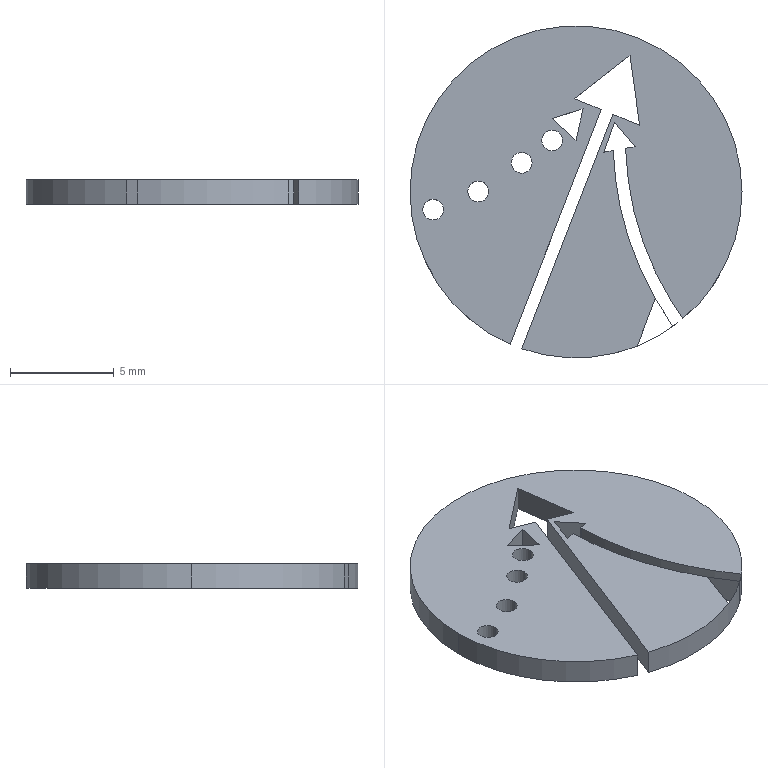Part | STEP file | Part 11_1 | 1 solid | 31 faces | box 16 x 16 x 1.2 mm | volume 213.852 mm3 | plane 17 | cylinder 12 | spline 2 | commonest cylinder face diameters 1 x8 16 x4
STEP:
#1=CARTESIAN_POINT('',(-6.382,-0.8597,1.2));
#2=VERTEX_POINT('',#1);
#3=CARTESIAN_POINT('',(-7.382,-0.8597,1.2));
#4=VERTEX_POINT('',#3);
#5=CARTESIAN_POINT('',(-6.882,-0.8597,1.2));
#6=DIRECTION('',(0.,0.,-1.));
#7=DIRECTION('',(-1.,0.,0.));
#8=AXIS2_PLACEMENT_3D('',#5,#6,#7);
#9=CIRCLE('',#8,0.5);
#10=EDGE_CURVE('',#2,#4,#9,.T.);
#11=ORIENTED_EDGE('',*,*,#10,.F.);
#12=CARTESIAN_POINT('',(-6.382,-0.8597,0.));
#13=VERTEX_POINT('',#12);
#14=CARTESIAN_POINT('',(-6.382,-0.8597,10.));
#15=DIRECTION('',(0.,0.,-1.));
#16=VECTOR('',#15,1000.);
#17=LINE('',#14,#16);
#18=EDGE_CURVE('',#2,#13,#17,.T.);
#19=ORIENTED_EDGE('',*,*,#18,.T.);
#20=CARTESIAN_POINT('',(-7.382,-0.8597,0.));
#21=VERTEX_POINT('',#20);
#22=CARTESIAN_POINT('',(-6.882,-0.8597,0.));
#23=DIRECTION('',(0.,0.,1.));
#24=DIRECTION('',(-1.,0.,0.));
#25=AXIS2_PLACEMENT_3D('',#22,#23,#24);
#26=CIRCLE('',#25,0.5);
#27=EDGE_CURVE('',#21,#13,#26,.T.);
#28=ORIENTED_EDGE('',*,*,#27,.F.);
#29=CARTESIAN_POINT('',(-7.382,-0.8597,10.));
#30=DIRECTION('',(0.,0.,-1.));
#31=VECTOR('',#30,1000.);
#32=LINE('',#29,#31);
#33=EDGE_CURVE('',#4,#21,#32,.T.);
#34=ORIENTED_EDGE('',*,*,#33,.F.);
#35=EDGE_LOOP('',(#11,#19,#28,#34));
#36=FACE_OUTER_BOUND('',#35,.T.);
#37=CARTESIAN_POINT('',(-6.882,-0.8597,10.));
#38=DIRECTION('',(0.,0.,-1.));
#39=DIRECTION('',(-1.,0.,0.));
#40=AXIS2_PLACEMENT_3D('',#37,#38,#39);
#41=CYLINDRICAL_SURFACE('',#40,0.5);
#42=ADVANCED_FACE('',(#36),#41,.F.);
#43=CARTESIAN_POINT('',(-2.114,1.401,1.2));
#44=VERTEX_POINT('',#43);
#45=CARTESIAN_POINT('',(-3.114,1.401,1.2));
#46=VERTEX_POINT('',#45);
#47=CARTESIAN_POINT('',(-2.614,1.401,1.2));
#48=DIRECTION('',(0.,0.,-1.));
#49=DIRECTION('',(-1.,0.,0.));
#50=AXIS2_PLACEMENT_3D('',#47,#48,#49);
#51=CIRCLE('',#50,0.5);
#52=EDGE_CURVE('',#44,#46,#51,.T.);
#53=ORIENTED_EDGE('',*,*,#52,.F.);
#54=CARTESIAN_POINT('',(-2.114,1.401,0.));
#55=VERTEX_POINT('',#54);
#56=CARTESIAN_POINT('',(-2.114,1.401,10.));
#57=DIRECTION('',(0.,0.,-1.));
#58=VECTOR('',#57,1000.);
#59=LINE('',#56,#58);
#60=EDGE_CURVE('',#44,#55,#59,.T.);
#61=ORIENTED_EDGE('',*,*,#60,.T.);
#62=CARTESIAN_POINT('',(-3.114,1.401,0.));
#63=VERTEX_POINT('',#62);
#64=CARTESIAN_POINT('',(-2.614,1.401,0.));
#65=DIRECTION('',(0.,0.,1.));
#66=DIRECTION('',(-1.,0.,0.));
#67=AXIS2_PLACEMENT_3D('',#64,#65,#66);
#68=CIRCLE('',#67,0.5);
#69=EDGE_CURVE('',#63,#55,#68,.T.);
#70=ORIENTED_EDGE('',*,*,#69,.F.);
#71=CARTESIAN_POINT('',(-3.114,1.401,10.));
#72=DIRECTION('',(0.,0.,-1.));
#73=VECTOR('',#72,1000.);
#74=LINE('',#71,#73);
#75=EDGE_CURVE('',#46,#63,#74,.T.);
#76=ORIENTED_EDGE('',*,*,#75,.F.);
#77=EDGE_LOOP('',(#53,#61,#70,#76));
#78=FACE_OUTER_BOUND('',#77,.T.);
#79=CARTESIAN_POINT('',(-2.614,1.401,10.));
#80=DIRECTION('',(0.,0.,-1.));
#81=DIRECTION('',(-1.,0.,0.));
#82=AXIS2_PLACEMENT_3D('',#79,#80,#81);
#83=CYLINDRICAL_SURFACE('',#82,0.5);
#84=ADVANCED_FACE('',(#78),#83,.F.);
#85=CARTESIAN_POINT('',(8.,0.,1.2));
#86=VERTEX_POINT('',#85);
#87=CARTESIAN_POINT('',(-8.,0.,1.2));
#88=VERTEX_POINT('',#87);
#89=CARTESIAN_POINT('',(0.,0.,1.2));
#90=DIRECTION('',(0.,0.,1.));
#91=DIRECTION('',(-1.,0.,0.));
#92=AXIS2_PLACEMENT_3D('',#89,#90,#91);
#93=CIRCLE('',#92,8.);
#94=EDGE_CURVE('',#86,#88,#93,.T.);
#95=ORIENTED_EDGE('',*,*,#94,.F.);
#96=CARTESIAN_POINT('',(8.,0.,0.));
#97=VERTEX_POINT('',#96);
#98=CARTESIAN_POINT('',(8.,0.,1.2));
#99=DIRECTION('',(0.,0.,-1.));
#100=VECTOR('',#99,1000.);
#101=LINE('',#98,#100);
#102=EDGE_CURVE('',#86,#97,#101,.T.);
#103=ORIENTED_EDGE('',*,*,#102,.T.);
#104=CARTESIAN_POINT('',(-8.,0.,0.));
#105=VERTEX_POINT('',#104);
#106=CARTESIAN_POINT('',(0.,0.,0.));
#107=DIRECTION('',(0.,0.,1.));
#108=DIRECTION('',(-1.,0.,0.));
#109=AXIS2_PLACEMENT_3D('',#106,#107,#108);
#110=CIRCLE('',#109,8.);
#111=EDGE_CURVE('',#97,#105,#110,.T.);
#112=ORIENTED_EDGE('',*,*,#111,.T.);
#113=CARTESIAN_POINT('',(-8.,0.,1.2));
#114=DIRECTION('',(0.,0.,-1.));
#115=VECTOR('',#114,1000.);
#116=LINE('',#113,#115);
#117=EDGE_CURVE('',#88,#105,#116,.T.);
#118=ORIENTED_EDGE('',*,*,#117,.F.);
#119=EDGE_LOOP('',(#95,#103,#112,#118));
#120=FACE_OUTER_BOUND('',#119,.T.);
#121=CARTESIAN_POINT('',(0.,0.,1.2));
#122=DIRECTION('',(0.,0.,-1.));
#123=DIRECTION('',(-1.,0.,0.));
#124=AXIS2_PLACEMENT_3D('',#121,#122,#123);
#125=CYLINDRICAL_SURFACE('',#124,8.);
#126=ADVANCED_FACE('',(#120),#125,.T.);
#127=CARTESIAN_POINT('',(-3.173,-7.344,1.2));
#128=VERTEX_POINT('',#127);
#129=CARTESIAN_POINT('',(0.,0.,1.2));
#130=DIRECTION('',(0.,0.,1.));
#131=DIRECTION('',(-1.,0.,0.));
#132=AXIS2_PLACEMENT_3D('',#129,#130,#131);
#133=CIRCLE('',#132,8.);
#134=EDGE_CURVE('',#88,#128,#133,.T.);
#135=ORIENTED_EDGE('',*,*,#134,.F.);
#136=ORIENTED_EDGE('',*,*,#117,.T.);
#137=CARTESIAN_POINT('',(-3.173,-7.344,0.));
#138=VERTEX_POINT('',#137);
#139=CARTESIAN_POINT('',(0.,0.,0.));
#140=DIRECTION('',(0.,0.,1.));
#141=DIRECTION('',(-1.,0.,0.));
#142=AXIS2_PLACEMENT_3D('',#139,#140,#141);
#143=CIRCLE('',#142,8.);
#144=EDGE_CURVE('',#105,#138,#143,.T.);
#145=ORIENTED_EDGE('',*,*,#144,.T.);
#146=CARTESIAN_POINT('',(-3.173,-7.344,10.));
#147=DIRECTION('',(0.,0.,-1.));
#148=VECTOR('',#147,1000.);
#149=LINE('',#146,#148);
#150=EDGE_CURVE('',#128,#138,#149,.T.);
#151=ORIENTED_EDGE('',*,*,#150,.F.);
#152=EDGE_LOOP('',(#135,#136,#145,#151));
#153=FACE_OUTER_BOUND('',#152,.T.);
#154=CARTESIAN_POINT('',(0.,0.,1.2));
#155=DIRECTION('',(0.,0.,-1.));
#156=DIRECTION('',(-1.,0.,0.));
#157=AXIS2_PLACEMENT_3D('',#154,#155,#156);
#158=CYLINDRICAL_SURFACE('',#157,8.);
#159=ADVANCED_FACE('',(#153),#158,.T.);
#160=CARTESIAN_POINT('',(-0.6476,2.481,1.2));
#161=VERTEX_POINT('',#160);
#162=CARTESIAN_POINT('',(-1.648,2.481,1.2));
#163=VERTEX_POINT('',#162);
#164=CARTESIAN_POINT('',(-1.148,2.481,1.2));
#165=DIRECTION('',(0.,0.,-1.));
#166=DIRECTION('',(-1.,0.,0.));
#167=AXIS2_PLACEMENT_3D('',#164,#165,#166);
#168=CIRCLE('',#167,0.5);
#169=EDGE_CURVE('',#161,#163,#168,.T.);
#170=ORIENTED_EDGE('',*,*,#169,.F.);
#171=CARTESIAN_POINT('',(-0.6476,2.481,0.));
#172=VERTEX_POINT('',#171);
#173=CARTESIAN_POINT('',(-0.6476,2.481,10.));
#174=DIRECTION('',(0.,0.,-1.));
#175=VECTOR('',#174,1000.);
#176=LINE('',#173,#175);
#177=EDGE_CURVE('',#161,#172,#176,.T.);
#178=ORIENTED_EDGE('',*,*,#177,.T.);
#179=CARTESIAN_POINT('',(-1.648,2.481,0.));
#180=VERTEX_POINT('',#179);
#181=CARTESIAN_POINT('',(-1.148,2.481,0.));
#182=DIRECTION('',(0.,0.,1.));
#183=DIRECTION('',(-1.,0.,0.));
#184=AXIS2_PLACEMENT_3D('',#181,#182,#183);
#185=CIRCLE('',#184,0.5);
#186=EDGE_CURVE('',#180,#172,#185,.T.);
#187=ORIENTED_EDGE('',*,*,#186,.F.);
#188=CARTESIAN_POINT('',(-1.648,2.481,10.));
#189=DIRECTION('',(0.,0.,-1.));
#190=VECTOR('',#189,1000.);
#191=LINE('',#188,#190);
#192=EDGE_CURVE('',#163,#180,#191,.T.);
#193=ORIENTED_EDGE('',*,*,#192,.F.);
#194=EDGE_LOOP('',(#170,#178,#187,#193));
#195=FACE_OUTER_BOUND('',#194,.T.);
#196=CARTESIAN_POINT('',(-1.148,2.481,10.));
#197=DIRECTION('',(0.,0.,-1.));
#198=DIRECTION('',(-1.,0.,0.));
#199=AXIS2_PLACEMENT_3D('',#196,#197,#198);
#200=CYLINDRICAL_SURFACE('',#199,0.5);
#201=ADVANCED_FACE('',(#195),#200,.F.);
#202=CARTESIAN_POINT('',(-4.212,0.01623,1.2));
#203=VERTEX_POINT('',#202);
#204=CARTESIAN_POINT('',(-5.212,0.01623,1.2));
#205=VERTEX_POINT('',#204);
#206=CARTESIAN_POINT('',(-4.712,0.01623,1.2));
#207=DIRECTION('',(0.,0.,-1.));
#208=DIRECTION('',(-1.,0.,0.));
#209=AXIS2_PLACEMENT_3D('',#206,#207,#208);
#210=CIRCLE('',#209,0.5);
#211=EDGE_CURVE('',#203,#205,#210,.T.);
#212=ORIENTED_EDGE('',*,*,#211,.F.);
#213=CARTESIAN_POINT('',(-4.212,0.01623,0.));
#214=VERTEX_POINT('',#213);
#215=CARTESIAN_POINT('',(-4.212,0.01623,10.));
#216=DIRECTION('',(0.,0.,-1.));
#217=VECTOR('',#216,1000.);
#218=LINE('',#215,#217);
#219=EDGE_CURVE('',#203,#214,#218,.T.);
#220=ORIENTED_EDGE('',*,*,#219,.T.);
#221=CARTESIAN_POINT('',(-5.212,0.01623,0.));
#222=VERTEX_POINT('',#221);
#223=CARTESIAN_POINT('',(-4.712,0.01623,0.));
#224=DIRECTION('',(0.,0.,1.));
#225=DIRECTION('',(-1.,0.,0.));
#226=AXIS2_PLACEMENT_3D('',#223,#224,#225);
#227=CIRCLE('',#226,0.5);
#228=EDGE_CURVE('',#222,#214,#227,.T.);
#229=ORIENTED_EDGE('',*,*,#228,.F.);
#230=CARTESIAN_POINT('',(-5.212,0.01623,10.));
#231=DIRECTION('',(0.,0.,-1.));
#232=VECTOR('',#231,1000.);
#233=LINE('',#230,#232);
#234=EDGE_CURVE('',#205,#222,#233,.T.);
#235=ORIENTED_EDGE('',*,*,#234,.F.);
#236=EDGE_LOOP('',(#212,#220,#229,#235));
#237=FACE_OUTER_BOUND('',#236,.T.);
#238=CARTESIAN_POINT('',(-4.712,0.01623,10.));
#239=DIRECTION('',(0.,0.,-1.));
#240=DIRECTION('',(-1.,0.,0.));
#241=AXIS2_PLACEMENT_3D('',#238,#239,#240);
#242=CYLINDRICAL_SURFACE('',#241,0.5);
#243=ADVANCED_FACE('',(#237),#242,.F.);
#244=CARTESIAN_POINT('',(-6.882,-0.8597,1.2));
#245=DIRECTION('',(0.,0.,-1.));
#246=DIRECTION('',(-1.,0.,0.));
#247=AXIS2_PLACEMENT_3D('',#244,#245,#246);
#248=CIRCLE('',#247,0.5);
#249=EDGE_CURVE('',#4,#2,#248,.T.);
#250=ORIENTED_EDGE('',*,*,#249,.T.);
#251=ORIENTED_EDGE('',*,*,#10,.T.);
#252=EDGE_LOOP('',(#250,#251));
#253=FACE_BOUND('',#252,.T.);
#254=CARTESIAN_POINT('',(-2.614,1.401,1.2));
#255=DIRECTION('',(0.,0.,-1.));
#256=DIRECTION('',(-1.,0.,0.));
#257=AXIS2_PLACEMENT_3D('',#254,#255,#256);
#258=CIRCLE('',#257,0.5);
#259=EDGE_CURVE('',#46,#44,#258,.T.);
#260=ORIENTED_EDGE('',*,*,#259,.T.);
#261=ORIENTED_EDGE('',*,*,#52,.T.);
#262=EDGE_LOOP('',(#260,#261));
#263=FACE_BOUND('',#262,.T.);
#264=CARTESIAN_POINT('',(0.0009448,2.481,1.2));
#265=VERTEX_POINT('',#264);
#266=CARTESIAN_POINT('',(-1.148,3.535,1.2));
#267=VERTEX_POINT('',#266);
#268=CARTESIAN_POINT('',(0.0009448,2.481,1.2));
#269=DIRECTION('',(-0.7368,0.6761,0.));
#270=VECTOR('',#269,1000.);
#271=LINE('',#268,#270);
#272=EDGE_CURVE('',#265,#267,#271,.T.);
#273=ORIENTED_EDGE('',*,*,#272,.T.);
#274=CARTESIAN_POINT('',(0.3395,4.003,1.2));
#275=VERTEX_POINT('',#274);
#276=CARTESIAN_POINT('',(-1.148,3.535,1.2));
#277=DIRECTION('',(0.9539,0.3,0.));
#278=VECTOR('',#277,1000.);
#279=LINE('',#276,#278);
#280=EDGE_CURVE('',#267,#275,#279,.T.);
#281=ORIENTED_EDGE('',*,*,#280,.T.);
#282=CARTESIAN_POINT('',(0.3395,4.003,1.2));
#283=DIRECTION('',(-0.2172,-0.9761,0.));
#284=VECTOR('',#283,1000.);
#285=LINE('',#282,#284);
#286=EDGE_CURVE('',#275,#265,#285,.T.);
#287=ORIENTED_EDGE('',*,*,#286,.T.);
#288=EDGE_LOOP('',(#273,#281,#287));
#289=FACE_BOUND('',#288,.T.);
#290=CARTESIAN_POINT('',(1.857,3.356,1.2));
#291=VERTEX_POINT('',#290);
#292=CARTESIAN_POINT('',(2.848,2.178,1.2));
#293=VERTEX_POINT('',#292);
#294=CARTESIAN_POINT('',(1.857,3.356,1.2));
#295=DIRECTION('',(0.6439,-0.7651,0.));
#296=VECTOR('',#295,1000.);
#297=LINE('',#294,#296);
#298=EDGE_CURVE('',#291,#293,#297,.T.);
#299=ORIENTED_EDGE('',*,*,#298,.T.);
#300=CARTESIAN_POINT('',(2.388,2.097,1.2));
#301=VERTEX_POINT('',#300);
#302=CARTESIAN_POINT('',(2.848,2.178,1.2));
#303=DIRECTION('',(-0.9845,-0.1751,0.));
#304=VECTOR('',#303,1000.);
#305=LINE('',#302,#304);
#306=EDGE_CURVE('',#293,#301,#305,.T.);
#307=ORIENTED_EDGE('',*,*,#306,.T.);
#308=CARTESIAN_POINT('',(2.39,2.055,1.2));
#309=VERTEX_POINT('',#308);
#310=CARTESIAN_POINT('',(2.388,2.097,1.2));
#311=DIRECTION('',(0.03649,-0.9993,0.));
#312=VECTOR('',#311,1000.);
#313=LINE('',#310,#312);
#314=EDGE_CURVE('',#301,#309,#313,.T.);
#315=ORIENTED_EDGE('',*,*,#314,.T.);
#316=CARTESIAN_POINT('',(5.148,-6.124,1.2));
#317=VERTEX_POINT('',#316);
#318=CARTESIAN_POINT('',(2.39,2.055,1.2));
#319=CARTESIAN_POINT('',(2.417,1.322,1.2));
#320=CARTESIAN_POINT('',(2.573,-0.1545,1.2));
#321=CARTESIAN_POINT('',(3.114,-2.242,1.2));
#322=CARTESIAN_POINT('',(3.95,-4.232,1.2));
#323=CARTESIAN_POINT('',(4.726,-5.519,1.2));
#324=CARTESIAN_POINT('',(5.148,-6.124,1.2));
#325=B_SPLINE_CURVE_WITH_KNOTS('',3,(#318,#319,#320,#321,#322,#323,#324),.UNSPECIFIED.,.F.,.F.,(4,1,1,1,4),(0.,0.002195,0.00439,0.006585,0.00876),.UNSPECIFIED.);
#326=EDGE_CURVE('',#309,#317,#325,.T.);
#327=ORIENTED_EDGE('',*,*,#326,.T.);
#328=CARTESIAN_POINT('',(0.,0.,1.2));
#329=DIRECTION('',(0.,0.,1.));
#330=DIRECTION('',(-1.,0.,0.));
#331=AXIS2_PLACEMENT_3D('',#328,#329,#330);
#332=CIRCLE('',#331,8.);
#333=EDGE_CURVE('',#317,#86,#332,.T.);
#334=ORIENTED_EDGE('',*,*,#333,.T.);
#335=ORIENTED_EDGE('',*,*,#94,.T.);
#336=ORIENTED_EDGE('',*,*,#134,.T.);
#337=CARTESIAN_POINT('',(1.217,3.963,1.2));
#338=VERTEX_POINT('',#337);
#339=CARTESIAN_POINT('',(-3.173,-7.344,1.2));
#340=DIRECTION('',(0.3619,0.9322,0.));
#341=VECTOR('',#340,1000.);
#342=LINE('',#339,#341);
#343=EDGE_CURVE('',#128,#338,#342,.T.);
#344=ORIENTED_EDGE('',*,*,#343,.T.);
#345=CARTESIAN_POINT('',(-0.07766,4.489,1.2));
#346=VERTEX_POINT('',#345);
#347=CARTESIAN_POINT('',(1.217,3.963,1.2));
#348=DIRECTION('',(-0.9262,0.377,0.));
#349=VECTOR('',#348,1000.);
#350=LINE('',#347,#349);
#351=EDGE_CURVE('',#338,#346,#350,.T.);
#352=ORIENTED_EDGE('',*,*,#351,.T.);
#353=CARTESIAN_POINT('',(2.603,6.573,1.2));
#354=VERTEX_POINT('',#353);
#355=CARTESIAN_POINT('',(-0.07766,4.489,1.2));
#356=DIRECTION('',(0.7896,0.6137,0.));
#357=VECTOR('',#356,1000.);
#358=LINE('',#355,#357);
#359=EDGE_CURVE('',#346,#354,#358,.T.);
#360=ORIENTED_EDGE('',*,*,#359,.T.);
#361=CARTESIAN_POINT('',(3.067,3.21,1.2));
#362=VERTEX_POINT('',#361);
#363=CARTESIAN_POINT('',(2.603,6.573,1.2));
#364=DIRECTION('',(0.1366,-0.9906,0.));
#365=VECTOR('',#364,1000.);
#366=LINE('',#363,#365);
#367=EDGE_CURVE('',#354,#362,#366,.T.);
#368=ORIENTED_EDGE('',*,*,#367,.T.);
#369=CARTESIAN_POINT('',(1.772,3.736,1.2));
#370=VERTEX_POINT('',#369);
#371=CARTESIAN_POINT('',(3.067,3.21,1.2));
#372=DIRECTION('',(-0.9262,0.377,0.));
#373=VECTOR('',#372,1000.);
#374=LINE('',#371,#373);
#375=EDGE_CURVE('',#362,#370,#374,.T.);
#376=ORIENTED_EDGE('',*,*,#375,.T.);
#377=CARTESIAN_POINT('',(-2.614,-7.561,1.2));
#378=VERTEX_POINT('',#377);
#379=CARTESIAN_POINT('',(1.772,3.736,1.2));
#380=DIRECTION('',(-0.3619,-0.9322,0.));
#381=VECTOR('',#380,1000.);
#382=LINE('',#379,#381);
#383=EDGE_CURVE('',#370,#378,#382,.T.);
#384=ORIENTED_EDGE('',*,*,#383,.T.);
#385=CARTESIAN_POINT('',(4.914,-6.313,1.2));
#386=VERTEX_POINT('',#385);
#387=CARTESIAN_POINT('',(0.,0.,1.2));
#388=DIRECTION('',(0.,0.,1.));
#389=DIRECTION('',(-1.,0.,0.));
#390=AXIS2_PLACEMENT_3D('',#387,#388,#389);
#391=CIRCLE('',#390,8.);
#392=EDGE_CURVE('',#378,#386,#391,.T.);
#393=ORIENTED_EDGE('',*,*,#392,.T.);
#394=CARTESIAN_POINT('',(4.668,-6.485,1.2));
#395=VERTEX_POINT('',#394);
#396=CARTESIAN_POINT('',(4.914,-6.313,1.2));
#397=DIRECTION('',(-0.8195,-0.573,0.));
#398=VECTOR('',#397,1000.);
#399=LINE('',#396,#398);
#400=EDGE_CURVE('',#386,#395,#399,.T.);
#401=ORIENTED_EDGE('',*,*,#400,.T.);
#402=CARTESIAN_POINT('',(1.792,1.991,1.2));
#403=VERTEX_POINT('',#402);
#404=CARTESIAN_POINT('',(4.668,-6.485,1.2));
#405=CARTESIAN_POINT('',(4.226,-5.852,1.2));
#406=CARTESIAN_POINT('',(3.417,-4.513,1.2));
#407=CARTESIAN_POINT('',(2.543,-2.435,1.2));
#408=CARTESIAN_POINT('',(1.984,-0.2741,1.2));
#409=CARTESIAN_POINT('',(1.821,1.243,1.2));
#410=CARTESIAN_POINT('',(1.792,1.991,1.2));
#411=B_SPLINE_CURVE_WITH_KNOTS('',3,(#404,#405,#406,#407,#408,#409,#410),.UNSPECIFIED.,.F.,.F.,(4,1,1,1,4),(0.,0.002283,0.004566,0.006849,0.009089),.UNSPECIFIED.);
#412=EDGE_CURVE('',#395,#403,#411,.T.);
#413=ORIENTED_EDGE('',*,*,#412,.T.);
#414=CARTESIAN_POINT('',(1.333,1.909,1.2));
#415=VERTEX_POINT('',#414);
#416=CARTESIAN_POINT('',(1.792,1.991,1.2));
#417=DIRECTION('',(-0.9845,-0.1751,0.));
#418=VECTOR('',#417,1000.);
#419=LINE('',#416,#418);
#420=EDGE_CURVE('',#403,#415,#419,.T.);
#421=ORIENTED_EDGE('',*,*,#420,.T.);
#422=CARTESIAN_POINT('',(1.333,1.909,1.2));
#423=DIRECTION('',(0.3406,0.9402,0.));
#424=VECTOR('',#423,1000.);
#425=LINE('',#422,#424);
#426=EDGE_CURVE('',#415,#291,#425,.T.);
#427=ORIENTED_EDGE('',*,*,#426,.T.);
#428=EDGE_LOOP('',(#299,#307,#315,#327,#334,#335,#336,#344,#352,#360,#368,#376,#384,#393,#401,#413,#421,#427));
#429=FACE_OUTER_BOUND('',#428,.T.);
#430=CARTESIAN_POINT('',(-1.148,2.481,1.2));
#431=DIRECTION('',(0.,0.,-1.));
#432=DIRECTION('',(-1.,0.,0.));
#433=AXIS2_PLACEMENT_3D('',#430,#431,#432);
#434=CIRCLE('',#433,0.5);
#435=EDGE_CURVE('',#163,#161,#434,.T.);
#436=ORIENTED_EDGE('',*,*,#435,.T.);
#437=ORIENTED_EDGE('',*,*,#169,.T.);
#438=EDGE_LOOP('',(#436,#437));
#439=FACE_BOUND('',#438,.T.);
#440=CARTESIAN_POINT('',(-4.712,0.01623,1.2));
#441=DIRECTION('',(0.,0.,-1.));
#442=DIRECTION('',(-1.,0.,0.));
#443=AXIS2_PLACEMENT_3D('',#440,#441,#442);
#444=CIRCLE('',#443,0.5);
#445=EDGE_CURVE('',#205,#203,#444,.T.);
#446=ORIENTED_EDGE('',*,*,#445,.T.);
#447=ORIENTED_EDGE('',*,*,#211,.T.);
#448=EDGE_LOOP('',(#446,#447));
#449=FACE_BOUND('',#448,.T.);
#450=CARTESIAN_POINT('',(0.,0.,1.2));
#451=DIRECTION('',(0.,0.,1.));
#452=DIRECTION('',(1.,0.,0.));
#453=AXIS2_PLACEMENT_3D('',#450,#451,#452);
#454=PLANE('',#453);
#455=ADVANCED_FACE('',(#253,#263,#289,#429,#439,#449),#454,.T.);
#456=ORIENTED_EDGE('',*,*,#18,.F.);
#457=ORIENTED_EDGE('',*,*,#249,.F.);
#458=ORIENTED_EDGE('',*,*,#33,.T.);
#459=CARTESIAN_POINT('',(-6.882,-0.8597,0.));
#460=DIRECTION('',(0.,0.,1.));
#461=DIRECTION('',(-1.,0.,0.));
#462=AXIS2_PLACEMENT_3D('',#459,#460,#461);
#463=CIRCLE('',#462,0.5);
#464=EDGE_CURVE('',#13,#21,#463,.T.);
#465=ORIENTED_EDGE('',*,*,#464,.F.);
#466=EDGE_LOOP('',(#456,#457,#458,#465));
#467=FACE_OUTER_BOUND('',#466,.T.);
#468=CARTESIAN_POINT('',(-6.882,-0.8597,10.));
#469=DIRECTION('',(0.,0.,-1.));
#470=DIRECTION('',(-1.,0.,0.));
#471=AXIS2_PLACEMENT_3D('',#468,#469,#470);
#472=CYLINDRICAL_SURFACE('',#471,0.5);
#473=ADVANCED_FACE('',(#467),#472,.F.);
#474=ORIENTED_EDGE('',*,*,#60,.F.);
#475=ORIENTED_EDGE('',*,*,#259,.F.);
#476=ORIENTED_EDGE('',*,*,#75,.T.);
#477=CARTESIAN_POINT('',(-2.614,1.401,0.));
#478=DIRECTION('',(0.,0.,1.));
#479=DIRECTION('',(-1.,0.,0.));
#480=AXIS2_PLACEMENT_3D('',#477,#478,#479);
#481=CIRCLE('',#480,0.5);
#482=EDGE_CURVE('',#55,#63,#481,.T.);
#483=ORIENTED_EDGE('',*,*,#482,.F.);
#484=EDGE_LOOP('',(#474,#475,#476,#483));
#485=FACE_OUTER_BOUND('',#484,.T.);
#486=CARTESIAN_POINT('',(-2.614,1.401,10.));
#487=DIRECTION('',(0.,0.,-1.));
#488=DIRECTION('',(-1.,0.,0.));
#489=AXIS2_PLACEMENT_3D('',#486,#487,#488);
#490=CYLINDRICAL_SURFACE('',#489,0.5);
#491=ADVANCED_FACE('',(#485),#490,.F.);
#492=CARTESIAN_POINT('',(0.3395,4.003,0.));
#493=VERTEX_POINT('',#492);
#494=CARTESIAN_POINT('',(0.3395,4.003,10.));
#495=DIRECTION('',(0.,0.,1.));
#496=VECTOR('',#495,1000.);
#497=LINE('',#494,#496);
#498=EDGE_CURVE('',#493,#275,#497,.T.);
#499=ORIENTED_EDGE('',*,*,#498,.T.);
#500=ORIENTED_EDGE('',*,*,#280,.F.);
#501=CARTESIAN_POINT('',(-1.148,3.535,0.));
#502=VERTEX_POINT('',#501);
#503=CARTESIAN_POINT('',(-1.148,3.535,10.));
#504=DIRECTION('',(0.,0.,-1.));
#505=VECTOR('',#504,1000.);
#506=LINE('',#503,#505);
#507=EDGE_CURVE('',#267,#502,#506,.T.);
#508=ORIENTED_EDGE('',*,*,#507,.T.);
#509=CARTESIAN_POINT('',(0.3395,4.003,0.));
#510=DIRECTION('',(0.9539,0.3,0.));
#511=VECTOR('',#510,1000.);
#512=LINE('',#509,#511);
#513=EDGE_CURVE('',#502,#493,#512,.T.);
#514=ORIENTED_EDGE('',*,*,#513,.T.);
#515=EDGE_LOOP('',(#499,#500,#508,#514));
#516=FACE_OUTER_BOUND('',#515,.T.);
#517=CARTESIAN_POINT('',(0.3395,4.003,10.));
#518=DIRECTION('',(0.3,-0.9539,0.));
#519=DIRECTION('',(0.9539,0.3,0.));
#520=AXIS2_PLACEMENT_3D('',#517,#518,#519);
#521=PLANE('',#520);
#522=ADVANCED_FACE('',(#516),#521,.T.);
#523=ORIENTED_EDGE('',*,*,#507,.F.);
#524=ORIENTED_EDGE('',*,*,#272,.F.);
#525=CARTESIAN_POINT('',(0.0009448,2.481,0.));
#526=VERTEX_POINT('',#525);
#527=CARTESIAN_POINT('',(0.0009448,2.481,10.));
#528=DIRECTION('',(0.,0.,-1.));
#529=VECTOR('',#528,1000.);
#530=LINE('',#527,#529);
#531=EDGE_CURVE('',#265,#526,#530,.T.);
#532=ORIENTED_EDGE('',*,*,#531,.T.);
#533=CARTESIAN_POINT('',(-1.148,3.535,0.));
#534=DIRECTION('',(-0.7368,0.6761,0.));
#535=VECTOR('',#534,1000.);
#536=LINE('',#533,#535);
#537=EDGE_CURVE('',#526,#502,#536,.T.);
#538=ORIENTED_EDGE('',*,*,#537,.T.);
#539=EDGE_LOOP('',(#523,#524,#532,#538));
#540=FACE_OUTER_BOUND('',#539,.T.);
#541=CARTESIAN_POINT('',(-1.148,3.535,10.));
#542=DIRECTION('',(0.6761,0.7368,0.));
#543=DIRECTION('',(-0.7368,0.6761,0.));
#544=AXIS2_PLACEMENT_3D('',#541,#542,#543);
#545=PLANE('',#544);
#546=ADVANCED_FACE('',(#540),#545,.T.);
#547=ORIENTED_EDGE('',*,*,#531,.F.);
#548=ORIENTED_EDGE('',*,*,#286,.F.);
#549=ORIENTED_EDGE('',*,*,#498,.F.);
#550=CARTESIAN_POINT('',(0.0009448,2.481,0.));
#551=DIRECTION('',(-0.2172,-0.9761,0.));
#552=VECTOR('',#551,1000.);
#553=LINE('',#550,#552);
#554=EDGE_CURVE('',#493,#526,#553,.T.);
#555=ORIENTED_EDGE('',*,*,#554,.T.);
#556=EDGE_LOOP('',(#547,#548,#549,#555));
#557=FACE_OUTER_BOUND('',#556,.T.);
#558=CARTESIAN_POINT('',(0.0009448,2.481,10.));
#559=DIRECTION('',(-0.9761,0.2172,0.));
#560=DIRECTION('',(-0.2172,-0.9761,0.));
#561=AXIS2_PLACEMENT_3D('',#558,#559,#560);
#562=PLANE('',#561);
#563=ADVANCED_FACE('',(#557),#562,.T.);
#564=CARTESIAN_POINT('',(2.388,2.097,0.));
#565=VERTEX_POINT('',#564);
#566=CARTESIAN_POINT('',(2.388,2.097,10.));
#567=DIRECTION('',(0.,0.,1.));
#568=VECTOR('',#567,1000.);
#569=LINE('',#566,#568);
#570=EDGE_CURVE('',#565,#301,#569,.T.);
#571=ORIENTED_EDGE('',*,*,#570,.T.);
#572=ORIENTED_EDGE('',*,*,#306,.F.);
#573=CARTESIAN_POINT('',(2.848,2.178,0.));
#574=VERTEX_POINT('',#573);
#575=CARTESIAN_POINT('',(2.848,2.178,10.));
#576=DIRECTION('',(0.,0.,-1.));
#577=VECTOR('',#576,1000.);
#578=LINE('',#575,#577);
#579=EDGE_CURVE('',#293,#574,#578,.T.);
#580=ORIENTED_EDGE('',*,*,#579,.T.);
#581=CARTESIAN_POINT('',(2.388,2.097,0.));
#582=DIRECTION('',(-0.9845,-0.1751,0.));
#583=VECTOR('',#582,1000.);
#584=LINE('',#581,#583);
#585=EDGE_CURVE('',#574,#565,#584,.T.);
#586=ORIENTED_EDGE('',*,*,#585,.T.);
#587=EDGE_LOOP('',(#571,#572,#580,#586));
#588=FACE_OUTER_BOUND('',#587,.T.);
#589=CARTESIAN_POINT('',(2.388,2.097,10.));
#590=DIRECTION('',(-0.1751,0.9845,0.));
#591=DIRECTION('',(-0.9845,-0.1751,0.));
#592=AXIS2_PLACEMENT_3D('',#589,#590,#591);
#593=PLANE('',#592);
#594=ADVANCED_FACE('',(#588),#593,.T.);
#595=ORIENTED_EDGE('',*,*,#579,.F.);
#596=ORIENTED_EDGE('',*,*,#298,.F.);
#597=CARTESIAN_POINT('',(1.857,3.356,0.));
#598=VERTEX_POINT('',#597);
#599=CARTESIAN_POINT('',(1.857,3.356,10.));
#600=DIRECTION('',(0.,0.,-1.));
#601=VECTOR('',#600,1000.);
#602=LINE('',#599,#601);
#603=EDGE_CURVE('',#291,#598,#602,.T.);
#604=ORIENTED_EDGE('',*,*,#603,.T.);
#605=CARTESIAN_POINT('',(2.848,2.178,0.));
#606=DIRECTION('',(0.6439,-0.7651,0.));
#607=VECTOR('',#606,1000.);
#608=LINE('',#605,#607);
#609=EDGE_CURVE('',#598,#574,#608,.T.);
#610=ORIENTED_EDGE('',*,*,#609,.T.);
#611=EDGE_LOOP('',(#595,#596,#604,#610));
#612=FACE_OUTER_BOUND('',#611,.T.);
#613=CARTESIAN_POINT('',(2.848,2.178,10.));
#614=DIRECTION('',(-0.7651,-0.6439,0.));
#615=DIRECTION('',(0.6439,-0.7651,0.));
#616=AXIS2_PLACEMENT_3D('',#613,#614,#615);
#617=PLANE('',#616);
#618=ADVANCED_FACE('',(#612),#617,.T.);
#619=ORIENTED_EDGE('',*,*,#603,.F.);
#620=ORIENTED_EDGE('',*,*,#426,.F.);
#621=CARTESIAN_POINT('',(1.333,1.909,0.));
#622=VERTEX_POINT('',#621);
#623=CARTESIAN_POINT('',(1.333,1.909,10.));
#624=DIRECTION('',(0.,0.,-1.));
#625=VECTOR('',#624,1000.);
#626=LINE('',#623,#625);
#627=EDGE_CURVE('',#415,#622,#626,.T.);
#628=ORIENTED_EDGE('',*,*,#627,.T.);
#629=CARTESIAN_POINT('',(1.857,3.356,0.));
#630=DIRECTION('',(0.3406,0.9402,0.));
#631=VECTOR('',#630,1000.);
#632=LINE('',#629,#631);
#633=EDGE_CURVE('',#622,#598,#632,.T.);
#634=ORIENTED_EDGE('',*,*,#633,.T.);
#635=EDGE_LOOP('',(#619,#620,#628,#634));
#636=FACE_OUTER_BOUND('',#635,.T.);
#637=CARTESIAN_POINT('',(1.857,3.356,10.));
#638=DIRECTION('',(0.9402,-0.3406,0.));
#639=DIRECTION('',(0.3406,0.9402,0.));
#640=AXIS2_PLACEMENT_3D('',#637,#638,#639);
#641=PLANE('',#640);
#642=ADVANCED_FACE('',(#636),#641,.T.);
#643=ORIENTED_EDGE('',*,*,#627,.F.);
#644=ORIENTED_EDGE('',*,*,#420,.F.);
#645=CARTESIAN_POINT('',(1.792,1.991,0.));
#646=VERTEX_POINT('',#645);
#647=CARTESIAN_POINT('',(1.792,1.991,10.));
#648=DIRECTION('',(0.,0.,-1.));
#649=VECTOR('',#648,1000.);
#650=LINE('',#647,#649);
#651=EDGE_CURVE('',#403,#646,#650,.T.);
#652=ORIENTED_EDGE('',*,*,#651,.T.);
#653=CARTESIAN_POINT('',(1.333,1.909,0.));
#654=DIRECTION('',(-0.9845,-0.1751,0.));
#655=VECTOR('',#654,1000.);
#656=LINE('',#653,#655);
#657=EDGE_CURVE('',#646,#622,#656,.T.);
#658=ORIENTED_EDGE('',*,*,#657,.T.);
#659=EDGE_LOOP('',(#643,#644,#652,#658));
#660=FACE_OUTER_BOUND('',#659,.T.);
#661=CARTESIAN_POINT('',(1.333,1.909,10.));
#662=DIRECTION('',(-0.1751,0.9845,0.));
#663=DIRECTION('',(-0.9845,-0.1751,0.));
#664=AXIS2_PLACEMENT_3D('',#661,#662,#663);
#665=PLANE('',#664);
#666=ADVANCED_FACE('',(#660),#665,.T.);
#667=ORIENTED_EDGE('',*,*,#651,.F.);
#668=ORIENTED_EDGE('',*,*,#412,.F.);
#669=CARTESIAN_POINT('',(4.668,-6.485,0.));
#670=VERTEX_POINT('',#669);
#671=CARTESIAN_POINT('',(4.668,-6.485,0.6));
#672=DIRECTION('',(0.,0.,-1.));
#673=VECTOR('',#672,1000.);
#674=LINE('',#671,#673);
#675=EDGE_CURVE('',#395,#670,#674,.T.);
#676=ORIENTED_EDGE('',*,*,#675,.T.);
#677=CARTESIAN_POINT('',(4.668,-6.485,0.));
#678=CARTESIAN_POINT('',(4.226,-5.852,0.));
#679=CARTESIAN_POINT('',(3.417,-4.513,0.));
#680=CARTESIAN_POINT('',(2.543,-2.435,0.));
#681=CARTESIAN_POINT('',(1.984,-0.2741,0.));
#682=CARTESIAN_POINT('',(1.821,1.243,0.));
#683=CARTESIAN_POINT('',(1.792,1.991,0.));
#684=B_SPLINE_CURVE_WITH_KNOTS('',3,(#677,#678,#679,#680,#681,#682,#683),.UNSPECIFIED.,.F.,.F.,(4,1,1,1,4),(0.,0.002283,0.004566,0.006849,0.009089),.UNSPECIFIED.);
#685=EDGE_CURVE('',#670,#646,#684,.T.);
#686=ORIENTED_EDGE('',*,*,#685,.T.);
#687=EDGE_LOOP('',(#667,#668,#676,#686));
#688=FACE_OUTER_BOUND('',#687,.T.);
#689=CARTESIAN_POINT('',(1.788,2.082,1.2));
#690=CARTESIAN_POINT('',(1.788,2.082,0.));
#691=CARTESIAN_POINT('',(1.79,2.051,1.2));
#692=CARTESIAN_POINT('',(1.79,2.051,0.));
#693=CARTESIAN_POINT('',(1.791,2.021,1.2));
#694=CARTESIAN_POINT('',(1.791,2.021,0.));
#695=CARTESIAN_POINT('',(1.792,1.991,1.2));
#696=CARTESIAN_POINT('',(1.792,1.991,0.));
#697=CARTESIAN_POINT('',(1.821,1.243,1.2));
#698=CARTESIAN_POINT('',(1.821,1.243,0.));
#699=CARTESIAN_POINT('',(1.984,-0.2741,1.2));
#700=CARTESIAN_POINT('',(1.984,-0.2741,0.));
#701=CARTESIAN_POINT('',(2.543,-2.435,1.2));
#702=CARTESIAN_POINT('',(2.543,-2.435,0.));
#703=CARTESIAN_POINT('',(3.417,-4.513,1.2));
#704=CARTESIAN_POINT('',(3.417,-4.513,0.));
#705=CARTESIAN_POINT('',(4.226,-5.852,1.2));
#706=CARTESIAN_POINT('',(4.226,-5.852,0.));
#707=CARTESIAN_POINT('',(4.668,-6.485,1.2));
#708=CARTESIAN_POINT('',(4.668,-6.485,0.));
#709=B_SPLINE_SURFACE_WITH_KNOTS('',3,1,((#689,#690),(#691,#692),(#693,#694),(#695,#696),(#697,#698),(#699,#700),(#701,#702),(#703,#704),(#705,#706),(#707,#708)),.UNSPECIFIED.,.F.,.F.,.F.,(4,3,1,1,1,4),(2,2),(-0.005347,0.004607,0.25,0.5,0.75,1.),(0.,1.),.UNSPECIFIED.);
#710=ADVANCED_FACE('',(#688),#709,.T.);
#711=ORIENTED_EDGE('',*,*,#675,.F.);
#712=ORIENTED_EDGE('',*,*,#400,.F.);
#713=CARTESIAN_POINT('',(4.914,-6.313,0.));
#714=VERTEX_POINT('',#713);
#715=CARTESIAN_POINT('',(4.914,-6.313,10.));
#716=DIRECTION('',(0.,0.,-1.));
#717=VECTOR('',#716,1000.);
#718=LINE('',#715,#717);
#719=EDGE_CURVE('',#386,#714,#718,.T.);
#720=ORIENTED_EDGE('',*,*,#719,.T.);
#721=CARTESIAN_POINT('',(4.668,-6.485,0.));
#722=DIRECTION('',(-0.8195,-0.573,0.));
#723=VECTOR('',#722,1000.);
#724=LINE('',#721,#723);
#725=EDGE_CURVE('',#714,#670,#724,.T.);
#726=ORIENTED_EDGE('',*,*,#725,.T.);
#727=EDGE_LOOP('',(#711,#712,#720,#726));
#728=FACE_OUTER_BOUND('',#727,.T.);
#729=CARTESIAN_POINT('',(4.668,-6.485,10.));
#730=DIRECTION('',(-0.573,0.8195,0.));
#731=DIRECTION('',(-0.8195,-0.573,0.));
#732=AXIS2_PLACEMENT_3D('',#729,#730,#731);
#733=PLANE('',#732);
#734=ADVANCED_FACE('',(#728),#733,.T.);
#735=CARTESIAN_POINT('',(-2.614,-7.561,0.));
#736=VERTEX_POINT('',#735);
#737=CARTESIAN_POINT('',(-2.614,-7.561,1.2));
#738=DIRECTION('',(0.,0.,-1.));
#739=VECTOR('',#738,1000.);
#740=LINE('',#737,#739);
#741=EDGE_CURVE('',#378,#736,#740,.T.);
#742=ORIENTED_EDGE('',*,*,#741,.T.);
#743=CARTESIAN_POINT('',(0.,0.,0.));
#744=DIRECTION('',(0.,0.,1.));
#745=DIRECTION('',(-1.,0.,0.));
#746=AXIS2_PLACEMENT_3D('',#743,#744,#745);
#747=CIRCLE('',#746,8.);
#748=EDGE_CURVE('',#736,#714,#747,.T.);
#749=ORIENTED_EDGE('',*,*,#748,.T.);
#750=ORIENTED_EDGE('',*,*,#719,.F.);
#751=ORIENTED_EDGE('',*,*,#392,.F.);
#752=EDGE_LOOP('',(#742,#749,#750,#751));
#753=FACE_OUTER_BOUND('',#752,.T.);
#754=CARTESIAN_POINT('',(0.,0.,1.2));
#755=DIRECTION('',(0.,0.,-1.));
#756=DIRECTION('',(-1.,0.,0.));
#757=AXIS2_PLACEMENT_3D('',#754,#755,#756);
#758=CYLINDRICAL_SURFACE('',#757,8.);
#759=ADVANCED_FACE('',(#753),#758,.T.);
#760=ORIENTED_EDGE('',*,*,#741,.F.);
#761=ORIENTED_EDGE('',*,*,#383,.F.);
#762=CARTESIAN_POINT('',(1.772,3.736,0.));
#763=VERTEX_POINT('',#762);
#764=CARTESIAN_POINT('',(1.772,3.736,10.));
#765=DIRECTION('',(0.,0.,-1.));
#766=VECTOR('',#765,1000.);
#767=LINE('',#764,#766);
#768=EDGE_CURVE('',#370,#763,#767,.T.);
#769=ORIENTED_EDGE('',*,*,#768,.T.);
#770=CARTESIAN_POINT('',(1.772,3.736,0.));
#771=DIRECTION('',(-0.3619,-0.9322,0.));
#772=VECTOR('',#771,1000.);
#773=LINE('',#770,#772);
#774=EDGE_CURVE('',#763,#736,#773,.T.);
#775=ORIENTED_EDGE('',*,*,#774,.T.);
#776=EDGE_LOOP('',(#760,#761,#769,#775));
#777=FACE_OUTER_BOUND('',#776,.T.);
#778=CARTESIAN_POINT('',(1.772,3.736,10.));
#779=DIRECTION('',(-0.9322,0.3619,0.));
#780=DIRECTION('',(-0.3619,-0.9322,0.));
#781=AXIS2_PLACEMENT_3D('',#778,#779,#780);
#782=PLANE('',#781);
#783=ADVANCED_FACE('',(#777),#782,.T.);
#784=ORIENTED_EDGE('',*,*,#768,.F.);
#785=ORIENTED_EDGE('',*,*,#375,.F.);
#786=CARTESIAN_POINT('',(3.067,3.21,0.));
#787=VERTEX_POINT('',#786);
#788=CARTESIAN_POINT('',(3.067,3.21,10.));
#789=DIRECTION('',(0.,0.,-1.));
#790=VECTOR('',#789,1000.);
#791=LINE('',#788,#790);
#792=EDGE_CURVE('',#362,#787,#791,.T.);
#793=ORIENTED_EDGE('',*,*,#792,.T.);
#794=CARTESIAN_POINT('',(1.772,3.736,0.));
#795=DIRECTION('',(-0.9262,0.377,0.));
#796=VECTOR('',#795,1000.);
#797=LINE('',#794,#796);
#798=EDGE_CURVE('',#787,#763,#797,.T.);
#799=ORIENTED_EDGE('',*,*,#798,.T.);
#800=EDGE_LOOP('',(#784,#785,#793,#799));
#801=FACE_OUTER_BOUND('',#800,.T.);
#802=CARTESIAN_POINT('',(1.772,3.736,10.));
#803=DIRECTION('',(0.377,0.9262,0.));
#804=DIRECTION('',(-0.9262,0.377,0.));
#805=AXIS2_PLACEMENT_3D('',#802,#803,#804);
#806=PLANE('',#805);
#807=ADVANCED_FACE('',(#801),#806,.T.);
#808=ORIENTED_EDGE('',*,*,#792,.F.);
#809=ORIENTED_EDGE('',*,*,#367,.F.);
#810=CARTESIAN_POINT('',(2.603,6.573,0.));
#811=VERTEX_POINT('',#810);
#812=CARTESIAN_POINT('',(2.603,6.573,10.));
#813=DIRECTION('',(0.,0.,-1.));
#814=VECTOR('',#813,1000.);
#815=LINE('',#812,#814);
#816=EDGE_CURVE('',#354,#811,#815,.T.);
#817=ORIENTED_EDGE('',*,*,#816,.T.);
#818=CARTESIAN_POINT('',(3.067,3.21,0.));
#819=DIRECTION('',(0.1366,-0.9906,0.));
#820=VECTOR('',#819,1000.);
#821=LINE('',#818,#820);
#822=EDGE_CURVE('',#811,#787,#821,.T.);
#823=ORIENTED_EDGE('',*,*,#822,.T.);
#824=EDGE_LOOP('',(#808,#809,#817,#823));
#825=FACE_OUTER_BOUND('',#824,.T.);
#826=CARTESIAN_POINT('',(3.067,3.21,10.));
#827=DIRECTION('',(-0.9906,-0.1366,0.));
#828=DIRECTION('',(0.1366,-0.9906,0.));
#829=AXIS2_PLACEMENT_3D('',#826,#827,#828);
#830=PLANE('',#829);
#831=ADVANCED_FACE('',(#825),#830,.T.);
#832=ORIENTED_EDGE('',*,*,#816,.F.);
#833=ORIENTED_EDGE('',*,*,#359,.F.);
#834=CARTESIAN_POINT('',(-0.07766,4.489,0.));
#835=VERTEX_POINT('',#834);
#836=CARTESIAN_POINT('',(-0.07766,4.489,10.));
#837=DIRECTION('',(0.,0.,-1.));
#838=VECTOR('',#837,1000.);
#839=LINE('',#836,#838);
#840=EDGE_CURVE('',#346,#835,#839,.T.);
#841=ORIENTED_EDGE('',*,*,#840,.T.);
#842=CARTESIAN_POINT('',(2.603,6.573,0.));
#843=DIRECTION('',(0.7896,0.6137,0.));
#844=VECTOR('',#843,1000.);
#845=LINE('',#842,#844);
#846=EDGE_CURVE('',#835,#811,#845,.T.);
#847=ORIENTED_EDGE('',*,*,#846,.T.);
#848=EDGE_LOOP('',(#832,#833,#841,#847));
#849=FACE_OUTER_BOUND('',#848,.T.);
#850=CARTESIAN_POINT('',(2.603,6.573,10.));
#851=DIRECTION('',(0.6137,-0.7896,0.));
#852=DIRECTION('',(0.7896,0.6137,0.));
#853=AXIS2_PLACEMENT_3D('',#850,#851,#852);
#854=PLANE('',#853);
#855=ADVANCED_FACE('',(#849),#854,.T.);
#856=ORIENTED_EDGE('',*,*,#840,.F.);
#857=ORIENTED_EDGE('',*,*,#351,.F.);
#858=CARTESIAN_POINT('',(1.217,3.963,0.));
#859=VERTEX_POINT('',#858);
#860=CARTESIAN_POINT('',(1.217,3.963,10.));
#861=DIRECTION('',(0.,0.,-1.));
#862=VECTOR('',#861,1000.);
#863=LINE('',#860,#862);
#864=EDGE_CURVE('',#338,#859,#863,.T.);
#865=ORIENTED_EDGE('',*,*,#864,.T.);
#866=CARTESIAN_POINT('',(-0.07766,4.489,0.));
#867=DIRECTION('',(-0.9262,0.377,0.));
#868=VECTOR('',#867,1000.);
#869=LINE('',#866,#868);
#870=EDGE_CURVE('',#859,#835,#869,.T.);
#871=ORIENTED_EDGE('',*,*,#870,.T.);
#872=EDGE_LOOP('',(#856,#857,#865,#871));
#873=FACE_OUTER_BOUND('',#872,.T.);
#874=CARTESIAN_POINT('',(-0.07766,4.489,10.));
#875=DIRECTION('',(0.377,0.9262,0.));
#876=DIRECTION('',(-0.9262,0.377,0.));
#877=AXIS2_PLACEMENT_3D('',#874,#875,#876);
#878=PLANE('',#877);
#879=ADVANCED_FACE('',(#873),#878,.T.);
#880=ORIENTED_EDGE('',*,*,#864,.F.);
#881=ORIENTED_EDGE('',*,*,#343,.F.);
#882=ORIENTED_EDGE('',*,*,#150,.T.);
#883=CARTESIAN_POINT('',(1.217,3.963,0.));
#884=DIRECTION('',(0.3619,0.9322,0.));
#885=VECTOR('',#884,1000.);
#886=LINE('',#883,#885);
#887=EDGE_CURVE('',#138,#859,#886,.T.);
#888=ORIENTED_EDGE('',*,*,#887,.T.);
#889=EDGE_LOOP('',(#880,#881,#882,#888));
#890=FACE_OUTER_BOUND('',#889,.T.);
#891=CARTESIAN_POINT('',(1.217,3.963,10.));
#892=DIRECTION('',(0.9322,-0.3619,0.));
#893=DIRECTION('',(0.3619,0.9322,0.));
#894=AXIS2_PLACEMENT_3D('',#891,#892,#893);
#895=PLANE('',#894);
#896=ADVANCED_FACE('',(#890),#895,.T.);
#897=ORIENTED_EDGE('',*,*,#102,.F.);
#898=ORIENTED_EDGE('',*,*,#333,.F.);
#899=CARTESIAN_POINT('',(5.148,-6.124,0.));
#900=VERTEX_POINT('',#899);
#901=CARTESIAN_POINT('',(5.148,-6.124,1.2));
#902=DIRECTION('',(0.,0.,-1.));
#903=VECTOR('',#902,1000.);
#904=LINE('',#901,#903);
#905=EDGE_CURVE('',#317,#900,#904,.T.);
#906=ORIENTED_EDGE('',*,*,#905,.T.);
#907=CARTESIAN_POINT('',(0.,0.,0.));
#908=DIRECTION('',(0.,0.,1.));
#909=DIRECTION('',(-1.,0.,0.));
#910=AXIS2_PLACEMENT_3D('',#907,#908,#909);
#911=CIRCLE('',#910,8.);
#912=EDGE_CURVE('',#900,#97,#911,.T.);
#913=ORIENTED_EDGE('',*,*,#912,.T.);
#914=EDGE_LOOP('',(#897,#898,#906,#913));
#915=FACE_OUTER_BOUND('',#914,.T.);
#916=CARTESIAN_POINT('',(0.,0.,1.2));
#917=DIRECTION('',(0.,0.,-1.));
#918=DIRECTION('',(-1.,0.,0.));
#919=AXIS2_PLACEMENT_3D('',#916,#917,#918);
#920=CYLINDRICAL_SURFACE('',#919,8.);
#921=ADVANCED_FACE('',(#915),#920,.T.);
#922=ORIENTED_EDGE('',*,*,#905,.F.);
#923=ORIENTED_EDGE('',*,*,#326,.F.);
#924=CARTESIAN_POINT('',(2.39,2.055,0.));
#925=VERTEX_POINT('',#924);
#926=CARTESIAN_POINT('',(2.39,2.055,0.6));
#927=DIRECTION('',(0.,0.,-1.));
#928=VECTOR('',#927,1000.);
#929=LINE('',#926,#928);
#930=EDGE_CURVE('',#309,#925,#929,.T.);
#931=ORIENTED_EDGE('',*,*,#930,.T.);
#932=CARTESIAN_POINT('',(2.39,2.055,0.));
#933=CARTESIAN_POINT('',(2.417,1.322,0.));
#934=CARTESIAN_POINT('',(2.573,-0.1545,0.));
#935=CARTESIAN_POINT('',(3.114,-2.242,0.));
#936=CARTESIAN_POINT('',(3.95,-4.232,0.));
#937=CARTESIAN_POINT('',(4.726,-5.519,0.));
#938=CARTESIAN_POINT('',(5.148,-6.124,0.));
#939=B_SPLINE_CURVE_WITH_KNOTS('',3,(#932,#933,#934,#935,#936,#937,#938),.UNSPECIFIED.,.F.,.F.,(4,1,1,1,4),(0.,0.002195,0.00439,0.006585,0.00876),.UNSPECIFIED.);
#940=EDGE_CURVE('',#925,#900,#939,.T.);
#941=ORIENTED_EDGE('',*,*,#940,.T.);
#942=EDGE_LOOP('',(#922,#923,#931,#941));
#943=FACE_OUTER_BOUND('',#942,.T.);
#944=CARTESIAN_POINT('',(5.148,-6.124,1.2));
#945=CARTESIAN_POINT('',(5.148,-6.124,0.));
#946=CARTESIAN_POINT('',(4.726,-5.519,1.2));
#947=CARTESIAN_POINT('',(4.726,-5.519,0.));
#948=CARTESIAN_POINT('',(3.95,-4.232,1.2));
#949=CARTESIAN_POINT('',(3.95,-4.232,0.));
#950=CARTESIAN_POINT('',(3.114,-2.242,1.2));
#951=CARTESIAN_POINT('',(3.114,-2.242,0.));
#952=CARTESIAN_POINT('',(2.573,-0.1545,1.2));
#953=CARTESIAN_POINT('',(2.573,-0.1545,0.));
#954=CARTESIAN_POINT('',(2.417,1.322,1.2));
#955=CARTESIAN_POINT('',(2.417,1.322,0.));
#956=CARTESIAN_POINT('',(2.39,2.055,1.2));
#957=CARTESIAN_POINT('',(2.39,2.055,0.));
#958=B_SPLINE_SURFACE_WITH_KNOTS('',3,1,((#944,#945),(#946,#947),(#948,#949),(#950,#951),(#952,#953),(#954,#955),(#956,#957)),.UNSPECIFIED.,.F.,.F.,.F.,(4,1,1,1,4),(2,2),(0.002359,0.25,0.5,0.75,1.),(0.,1.),.UNSPECIFIED.);
#959=ADVANCED_FACE('',(#943),#958,.T.);
#960=ORIENTED_EDGE('',*,*,#930,.F.);
#961=ORIENTED_EDGE('',*,*,#314,.F.);
#962=ORIENTED_EDGE('',*,*,#570,.F.);
#963=CARTESIAN_POINT('',(2.39,2.055,0.));
#964=DIRECTION('',(0.03649,-0.9993,0.));
#965=VECTOR('',#964,1000.);
#966=LINE('',#963,#965);
#967=EDGE_CURVE('',#565,#925,#966,.T.);
#968=ORIENTED_EDGE('',*,*,#967,.T.);
#969=EDGE_LOOP('',(#960,#961,#962,#968));
#970=FACE_OUTER_BOUND('',#969,.T.);
#971=CARTESIAN_POINT('',(2.39,2.055,10.));
#972=DIRECTION('',(-0.9993,-0.03649,0.));
#973=DIRECTION('',(0.03649,-0.9993,0.));
#974=AXIS2_PLACEMENT_3D('',#971,#972,#973);
#975=PLANE('',#974);
#976=ADVANCED_FACE('',(#970),#975,.T.);
#977=ORIENTED_EDGE('',*,*,#177,.F.);
#978=ORIENTED_EDGE('',*,*,#435,.F.);
#979=ORIENTED_EDGE('',*,*,#192,.T.);
#980=CARTESIAN_POINT('',(-1.148,2.481,0.));
#981=DIRECTION('',(0.,0.,1.));
#982=DIRECTION('',(-1.,0.,0.));
#983=AXIS2_PLACEMENT_3D('',#980,#981,#982);
#984=CIRCLE('',#983,0.5);
#985=EDGE_CURVE('',#172,#180,#984,.T.);
#986=ORIENTED_EDGE('',*,*,#985,.F.);
#987=EDGE_LOOP('',(#977,#978,#979,#986));
#988=FACE_OUTER_BOUND('',#987,.T.);
#989=CARTESIAN_POINT('',(-1.148,2.481,10.));
#990=DIRECTION('',(0.,0.,-1.));
#991=DIRECTION('',(-1.,0.,0.));
#992=AXIS2_PLACEMENT_3D('',#989,#990,#991);
#993=CYLINDRICAL_SURFACE('',#992,0.5);
#994=ADVANCED_FACE('',(#988),#993,.F.);
#995=ORIENTED_EDGE('',*,*,#219,.F.);
#996=ORIENTED_EDGE('',*,*,#445,.F.);
#997=ORIENTED_EDGE('',*,*,#234,.T.);
#998=CARTESIAN_POINT('',(-4.712,0.01623,0.));
#999=DIRECTION('',(0.,0.,1.));
#1000=DIRECTION('',(-1.,0.,0.));
#1001=AXIS2_PLACEMENT_3D('',#998,#999,#1000);
#1002=CIRCLE('',#1001,0.5);
#1003=EDGE_CURVE('',#214,#222,#1002,.T.);
#1004=ORIENTED_EDGE('',*,*,#1003,.F.);
#1005=EDGE_LOOP('',(#995,#996,#997,#1004));
#1006=FACE_OUTER_BOUND('',#1005,.T.);
#1007=CARTESIAN_POINT('',(-4.712,0.01623,10.));
#1008=DIRECTION('',(0.,0.,-1.));
#1009=DIRECTION('',(-1.,0.,0.));
#1010=AXIS2_PLACEMENT_3D('',#1007,#1008,#1009);
#1011=CYLINDRICAL_SURFACE('',#1010,0.5);
#1012=ADVANCED_FACE('',(#1006),#1011,.F.);
#1013=ORIENTED_EDGE('',*,*,#27,.T.);
#1014=ORIENTED_EDGE('',*,*,#464,.T.);
#1015=EDGE_LOOP('',(#1013,#1014));
#1016=FACE_BOUND('',#1015,.T.);
#1017=ORIENTED_EDGE('',*,*,#69,.T.);
#1018=ORIENTED_EDGE('',*,*,#482,.T.);
#1019=EDGE_LOOP('',(#1017,#1018));
#1020=FACE_BOUND('',#1019,.T.);
#1021=ORIENTED_EDGE('',*,*,#554,.F.);
#1022=ORIENTED_EDGE('',*,*,#513,.F.);
#1023=ORIENTED_EDGE('',*,*,#537,.F.);
#1024=EDGE_LOOP('',(#1021,#1022,#1023));
#1025=FACE_BOUND('',#1024,.T.);
#1026=ORIENTED_EDGE('',*,*,#967,.F.);
#1027=ORIENTED_EDGE('',*,*,#585,.F.);
#1028=ORIENTED_EDGE('',*,*,#609,.F.);
#1029=ORIENTED_EDGE('',*,*,#633,.F.);
#1030=ORIENTED_EDGE('',*,*,#657,.F.);
#1031=ORIENTED_EDGE('',*,*,#685,.F.);
#1032=ORIENTED_EDGE('',*,*,#725,.F.);
#1033=ORIENTED_EDGE('',*,*,#748,.F.);
#1034=ORIENTED_EDGE('',*,*,#774,.F.);
#1035=ORIENTED_EDGE('',*,*,#798,.F.);
#1036=ORIENTED_EDGE('',*,*,#822,.F.);
#1037=ORIENTED_EDGE('',*,*,#846,.F.);
#1038=ORIENTED_EDGE('',*,*,#870,.F.);
#1039=ORIENTED_EDGE('',*,*,#887,.F.);
#1040=ORIENTED_EDGE('',*,*,#144,.F.);
#1041=ORIENTED_EDGE('',*,*,#111,.F.);
#1042=ORIENTED_EDGE('',*,*,#912,.F.);
#1043=ORIENTED_EDGE('',*,*,#940,.F.);
#1044=EDGE_LOOP('',(#1026,#1027,#1028,#1029,#1030,#1031,#1032,#1033,#1034,#1035,#1036,#1037,#1038,#1039,#1040,#1041,#1042,#1043));
#1045=FACE_OUTER_BOUND('',#1044,.T.);
#1046=ORIENTED_EDGE('',*,*,#186,.T.);
#1047=ORIENTED_EDGE('',*,*,#985,.T.);
#1048=EDGE_LOOP('',(#1046,#1047));
#1049=FACE_BOUND('',#1048,.T.);
#1050=ORIENTED_EDGE('',*,*,#228,.T.);
#1051=ORIENTED_EDGE('',*,*,#1003,.T.);
#1052=EDGE_LOOP('',(#1050,#1051));
#1053=FACE_BOUND('',#1052,.T.);
#1054=CARTESIAN_POINT('',(0.,0.,0.));
#1055=DIRECTION('',(0.,0.,1.));
#1056=DIRECTION('',(1.,0.,0.));
#1057=AXIS2_PLACEMENT_3D('',#1054,#1055,#1056);
#1058=PLANE('',#1057);
#1059=ADVANCED_FACE('',(#1016,#1020,#1025,#1045,#1049,#1053),#1058,.F.);
#1060=CLOSED_SHELL('',(#42,#84,#126,#159,#201,#243,#455,#473,#491,#522,#546,#563,#594,#618,#642,#666,#710,#734,#759,#783,#807,#831,#855,#879,#896,#921,#959,#976,#994,#1012,#1059));
#1061=MANIFOLD_SOLID_BREP('',#1060);
#1062=CARTESIAN_POINT('',(0.,0.,0.));
#1063=DIRECTION('',(0.,0.,1.));
#1064=DIRECTION('',(1.,0.,0.));
#1065=AXIS2_PLACEMENT_3D('',#1062,#1063,#1064);
#1066=(LENGTH_UNIT()NAMED_UNIT(*)SI_UNIT(.MILLI.,.METRE.));
#1067=UNCERTAINTY_MEASURE_WITH_UNIT(LENGTH_MEASURE(0.00001),#1066,'','');
#1068=(NAMED_UNIT(*)PLANE_ANGLE_UNIT()SI_UNIT($,.RADIAN.));
#1069=(NAMED_UNIT(*)SI_UNIT($,.STERADIAN.)SOLID_ANGLE_UNIT());
#1070=(GEOMETRIC_REPRESENTATION_CONTEXT(3)GLOBAL_UNCERTAINTY_ASSIGNED_CONTEXT((#1067))GLOBAL_UNIT_ASSIGNED_CONTEXT((#1066,#1068,#1069))REPRESENTATION_CONTEXT('',''));
#1071=ADVANCED_BREP_SHAPE_REPRESENTATION('',(#1061,#1065),#1070);